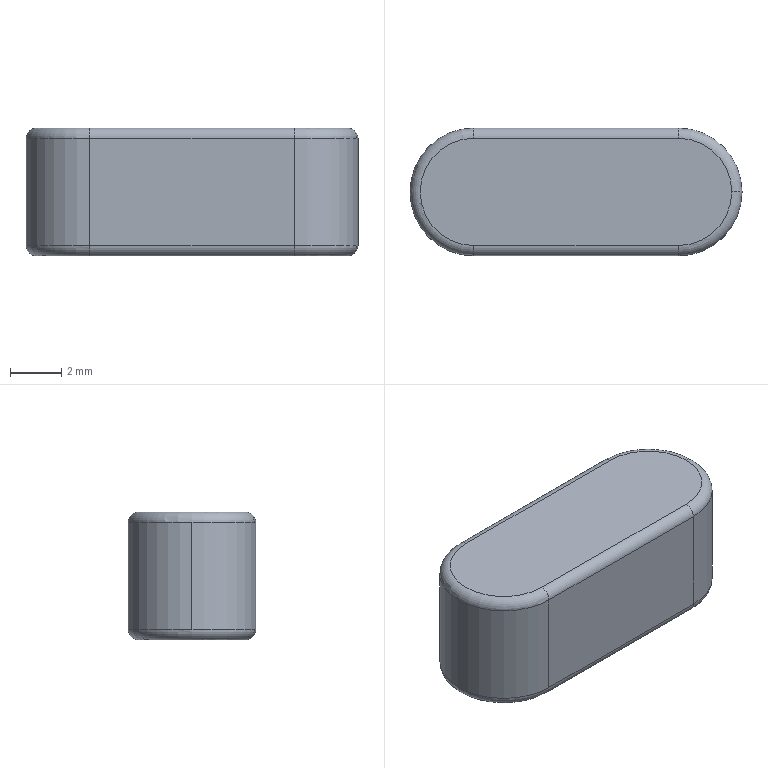Part | SolidWorks | features Extrusion 1, Fillet 1 | 1 solid | 17 faces | box 13 x 5 x 5 mm | volume 296.036 mm3 | cylinder 7 | torus 6 | plane 4 | commonest cylinder face diameters 0.8 x4 5 x3
STEP:
#1=CARTESIAN_POINT('',(6.1,0.,0.));
#2=VERTEX_POINT('',#1);
#3=CARTESIAN_POINT('',(4.,-2.1,0.));
#4=VERTEX_POINT('',#3);
#5=CARTESIAN_POINT('',(4.,0.,0.));
#6=DIRECTION('',(0.,0.,-1.));
#7=DIRECTION('',(1.,0.,0.));
#8=AXIS2_PLACEMENT_3D('',#5,#6,#7);
#9=CIRCLE('',#8,2.1);
#10=EDGE_CURVE('',#2,#4,#9,.T.);
#11=ORIENTED_EDGE('',*,*,#10,.F.);
#12=CARTESIAN_POINT('',(6.5,0.,0.4));
#13=VERTEX_POINT('',#12);
#14=CARTESIAN_POINT('',(6.1,0.,0.4));
#15=DIRECTION('',(0.,-1.,0.));
#16=DIRECTION('',(0.,0.,-1.));
#17=AXIS2_PLACEMENT_3D('',#14,#15,#16);
#18=CIRCLE('',#17,0.4);
#19=EDGE_CURVE('',#2,#13,#18,.T.);
#20=ORIENTED_EDGE('',*,*,#19,.T.);
#21=CARTESIAN_POINT('',(4.,-2.5,0.4));
#22=VERTEX_POINT('',#21);
#23=CARTESIAN_POINT('',(4.,0.,0.4));
#24=DIRECTION('',(0.,0.,1.));
#25=DIRECTION('',(1.,0.,0.));
#26=AXIS2_PLACEMENT_3D('',#23,#24,#25);
#27=CIRCLE('',#26,2.5);
#28=EDGE_CURVE('',#22,#13,#27,.T.);
#29=ORIENTED_EDGE('',*,*,#28,.F.);
#30=CARTESIAN_POINT('',(4.,-2.1,0.4));
#31=DIRECTION('',(1.,0.,0.));
#32=DIRECTION('',(0.,0.,-1.));
#33=AXIS2_PLACEMENT_3D('',#30,#31,#32);
#34=CIRCLE('',#33,0.4);
#35=EDGE_CURVE('',#22,#4,#34,.T.);
#36=ORIENTED_EDGE('',*,*,#35,.T.);
#37=EDGE_LOOP('',(#11,#20,#29,#36));
#38=FACE_OUTER_BOUND('',#37,.T.);
#39=CARTESIAN_POINT('',(4.,0.,0.4));
#40=DIRECTION('',(0.,0.,1.));
#41=DIRECTION('',(1.,0.,0.));
#42=AXIS2_PLACEMENT_3D('',#39,#40,#41);
#43=TOROIDAL_SURFACE('',#42,2.1,0.4);
#44=ADVANCED_FACE('',(#38),#43,.T.);
#45=CARTESIAN_POINT('',(6.5,0.,4.6));
#46=VERTEX_POINT('',#45);
#47=CARTESIAN_POINT('',(4.,-2.5,4.6));
#48=VERTEX_POINT('',#47);
#49=CARTESIAN_POINT('',(4.,0.,4.6));
#50=DIRECTION('',(0.,0.,-1.));
#51=DIRECTION('',(1.,0.,0.));
#52=AXIS2_PLACEMENT_3D('',#49,#50,#51);
#53=CIRCLE('',#52,2.5);
#54=EDGE_CURVE('',#46,#48,#53,.T.);
#55=ORIENTED_EDGE('',*,*,#54,.F.);
#56=CARTESIAN_POINT('',(6.1,0.,5.));
#57=VERTEX_POINT('',#56);
#58=CARTESIAN_POINT('',(6.1,0.,4.6));
#59=DIRECTION('',(0.,-1.,0.));
#60=DIRECTION('',(0.,0.,-1.));
#61=AXIS2_PLACEMENT_3D('',#58,#59,#60);
#62=CIRCLE('',#61,0.4);
#63=EDGE_CURVE('',#46,#57,#62,.T.);
#64=ORIENTED_EDGE('',*,*,#63,.T.);
#65=CARTESIAN_POINT('',(4.,-2.1,5.));
#66=VERTEX_POINT('',#65);
#67=CARTESIAN_POINT('',(4.,0.,5.));
#68=DIRECTION('',(0.,0.,1.));
#69=DIRECTION('',(1.,0.,0.));
#70=AXIS2_PLACEMENT_3D('',#67,#68,#69);
#71=CIRCLE('',#70,2.1);
#72=EDGE_CURVE('',#66,#57,#71,.T.);
#73=ORIENTED_EDGE('',*,*,#72,.F.);
#74=CARTESIAN_POINT('',(4.,-2.1,4.6));
#75=DIRECTION('',(1.,0.,0.));
#76=DIRECTION('',(0.,0.,-1.));
#77=AXIS2_PLACEMENT_3D('',#74,#75,#76);
#78=CIRCLE('',#77,0.4);
#79=EDGE_CURVE('',#66,#48,#78,.T.);
#80=ORIENTED_EDGE('',*,*,#79,.T.);
#81=EDGE_LOOP('',(#55,#64,#73,#80));
#82=FACE_OUTER_BOUND('',#81,.T.);
#83=CARTESIAN_POINT('',(4.,0.,4.6));
#84=DIRECTION('',(0.,0.,1.));
#85=DIRECTION('',(1.,0.,0.));
#86=AXIS2_PLACEMENT_3D('',#83,#84,#85);
#87=TOROIDAL_SURFACE('',#86,2.1,0.4);
#88=ADVANCED_FACE('',(#82),#87,.T.);
#89=CARTESIAN_POINT('',(-4.,-2.5,4.6));
#90=VERTEX_POINT('',#89);
#91=CARTESIAN_POINT('',(-6.5,0.,4.6));
#92=VERTEX_POINT('',#91);
#93=CARTESIAN_POINT('',(-4.,0.,4.6));
#94=DIRECTION('',(0.,0.,-1.));
#95=DIRECTION('',(1.,0.,0.));
#96=AXIS2_PLACEMENT_3D('',#93,#94,#95);
#97=CIRCLE('',#96,2.5);
#98=EDGE_CURVE('',#90,#92,#97,.T.);
#99=ORIENTED_EDGE('',*,*,#98,.T.);
#100=CARTESIAN_POINT('',(-6.5,0.,0.4));
#101=VERTEX_POINT('',#100);
#102=CARTESIAN_POINT('',(-6.5,0.,5.));
#103=DIRECTION('',(0.,0.,-1.));
#104=VECTOR('',#103,1000.);
#105=LINE('',#102,#104);
#106=EDGE_CURVE('',#92,#101,#105,.T.);
#107=ORIENTED_EDGE('',*,*,#106,.T.);
#108=CARTESIAN_POINT('',(-4.,-2.5,0.4));
#109=VERTEX_POINT('',#108);
#110=CARTESIAN_POINT('',(-4.,0.,0.4));
#111=DIRECTION('',(0.,0.,1.));
#112=DIRECTION('',(1.,0.,0.));
#113=AXIS2_PLACEMENT_3D('',#110,#111,#112);
#114=CIRCLE('',#113,2.5);
#115=EDGE_CURVE('',#101,#109,#114,.T.);
#116=ORIENTED_EDGE('',*,*,#115,.T.);
#117=CARTESIAN_POINT('',(-4.,-2.5,5.));
#118=DIRECTION('',(0.,0.,-1.));
#119=VECTOR('',#118,1000.);
#120=LINE('',#117,#119);
#121=EDGE_CURVE('',#90,#109,#120,.T.);
#122=ORIENTED_EDGE('',*,*,#121,.F.);
#123=EDGE_LOOP('',(#99,#107,#116,#122));
#124=FACE_OUTER_BOUND('',#123,.T.);
#125=CARTESIAN_POINT('',(-4.,0.,5.));
#126=DIRECTION('',(0.,0.,-1.));
#127=DIRECTION('',(-1.,0.,0.));
#128=AXIS2_PLACEMENT_3D('',#125,#126,#127);
#129=CYLINDRICAL_SURFACE('',#128,2.5);
#130=ADVANCED_FACE('',(#124),#129,.T.);
#131=ORIENTED_EDGE('',*,*,#106,.F.);
#132=CARTESIAN_POINT('',(-4.,2.5,4.6));
#133=VERTEX_POINT('',#132);
#134=CARTESIAN_POINT('',(-4.,0.,4.6));
#135=DIRECTION('',(0.,0.,-1.));
#136=DIRECTION('',(1.,0.,0.));
#137=AXIS2_PLACEMENT_3D('',#134,#135,#136);
#138=CIRCLE('',#137,2.5);
#139=EDGE_CURVE('',#92,#133,#138,.T.);
#140=ORIENTED_EDGE('',*,*,#139,.T.);
#141=CARTESIAN_POINT('',(-4.,2.5,0.4));
#142=VERTEX_POINT('',#141);
#143=CARTESIAN_POINT('',(-4.,2.5,5.));
#144=DIRECTION('',(0.,0.,-1.));
#145=VECTOR('',#144,1000.);
#146=LINE('',#143,#145);
#147=EDGE_CURVE('',#133,#142,#146,.T.);
#148=ORIENTED_EDGE('',*,*,#147,.T.);
#149=CARTESIAN_POINT('',(-4.,0.,0.4));
#150=DIRECTION('',(0.,0.,1.));
#151=DIRECTION('',(1.,0.,0.));
#152=AXIS2_PLACEMENT_3D('',#149,#150,#151);
#153=CIRCLE('',#152,2.5);
#154=EDGE_CURVE('',#142,#101,#153,.T.);
#155=ORIENTED_EDGE('',*,*,#154,.T.);
#156=EDGE_LOOP('',(#131,#140,#148,#155));
#157=FACE_OUTER_BOUND('',#156,.T.);
#158=CARTESIAN_POINT('',(-4.,0.,5.));
#159=DIRECTION('',(0.,0.,-1.));
#160=DIRECTION('',(-1.,0.,0.));
#161=AXIS2_PLACEMENT_3D('',#158,#159,#160);
#162=CYLINDRICAL_SURFACE('',#161,2.5);
#163=ADVANCED_FACE('',(#157),#162,.T.);
#164=CARTESIAN_POINT('',(4.,-2.5,5.));
#165=DIRECTION('',(0.,0.,-1.));
#166=VECTOR('',#165,1000.);
#167=LINE('',#164,#166);
#168=EDGE_CURVE('',#48,#22,#167,.T.);
#169=ORIENTED_EDGE('',*,*,#168,.F.);
#170=CARTESIAN_POINT('',(-4.,-2.5,4.6));
#171=DIRECTION('',(-1.,0.,0.));
#172=VECTOR('',#171,1000.);
#173=LINE('',#170,#172);
#174=EDGE_CURVE('',#48,#90,#173,.T.);
#175=ORIENTED_EDGE('',*,*,#174,.T.);
#176=ORIENTED_EDGE('',*,*,#121,.T.);
#177=CARTESIAN_POINT('',(-4.,-2.5,0.4));
#178=DIRECTION('',(1.,0.,0.));
#179=VECTOR('',#178,1000.);
#180=LINE('',#177,#179);
#181=EDGE_CURVE('',#109,#22,#180,.T.);
#182=ORIENTED_EDGE('',*,*,#181,.T.);
#183=EDGE_LOOP('',(#169,#175,#176,#182));
#184=FACE_OUTER_BOUND('',#183,.T.);
#185=CARTESIAN_POINT('',(-4.,-2.5,5.));
#186=DIRECTION('',(0.,1.,0.));
#187=DIRECTION('',(-1.,0.,0.));
#188=AXIS2_PLACEMENT_3D('',#185,#186,#187);
#189=PLANE('',#188);
#190=ADVANCED_FACE('',(#184),#189,.F.);
#191=CARTESIAN_POINT('',(4.,2.5,4.6));
#192=VERTEX_POINT('',#191);
#193=CARTESIAN_POINT('',(4.,2.5,0.4));
#194=VERTEX_POINT('',#193);
#195=CARTESIAN_POINT('',(4.,2.5,5.));
#196=DIRECTION('',(0.,0.,-1.));
#197=VECTOR('',#196,1000.);
#198=LINE('',#195,#197);
#199=EDGE_CURVE('',#192,#194,#198,.T.);
#200=ORIENTED_EDGE('',*,*,#199,.F.);
#201=CARTESIAN_POINT('',(4.,0.,4.6));
#202=DIRECTION('',(0.,0.,-1.));
#203=DIRECTION('',(1.,0.,0.));
#204=AXIS2_PLACEMENT_3D('',#201,#202,#203);
#205=CIRCLE('',#204,2.5);
#206=EDGE_CURVE('',#192,#46,#205,.T.);
#207=ORIENTED_EDGE('',*,*,#206,.T.);
#208=ORIENTED_EDGE('',*,*,#54,.T.);
#209=ORIENTED_EDGE('',*,*,#168,.T.);
#210=ORIENTED_EDGE('',*,*,#28,.T.);
#211=CARTESIAN_POINT('',(4.,0.,0.4));
#212=DIRECTION('',(0.,0.,1.));
#213=DIRECTION('',(1.,0.,0.));
#214=AXIS2_PLACEMENT_3D('',#211,#212,#213);
#215=CIRCLE('',#214,2.5);
#216=EDGE_CURVE('',#13,#194,#215,.T.);
#217=ORIENTED_EDGE('',*,*,#216,.T.);
#218=EDGE_LOOP('',(#200,#207,#208,#209,#210,#217));
#219=FACE_OUTER_BOUND('',#218,.T.);
#220=CARTESIAN_POINT('',(4.,0.,5.));
#221=DIRECTION('',(0.,0.,-1.));
#222=DIRECTION('',(-1.,0.,0.));
#223=AXIS2_PLACEMENT_3D('',#220,#221,#222);
#224=CYLINDRICAL_SURFACE('',#223,2.5);
#225=ADVANCED_FACE('',(#219),#224,.T.);
#226=ORIENTED_EDGE('',*,*,#147,.F.);
#227=CARTESIAN_POINT('',(4.,2.5,4.6));
#228=DIRECTION('',(1.,0.,0.));
#229=VECTOR('',#228,1000.);
#230=LINE('',#227,#229);
#231=EDGE_CURVE('',#133,#192,#230,.T.);
#232=ORIENTED_EDGE('',*,*,#231,.T.);
#233=ORIENTED_EDGE('',*,*,#199,.T.);
#234=CARTESIAN_POINT('',(-4.,2.5,0.4));
#235=DIRECTION('',(-1.,0.,0.));
#236=VECTOR('',#235,1000.);
#237=LINE('',#234,#236);
#238=EDGE_CURVE('',#194,#142,#237,.T.);
#239=ORIENTED_EDGE('',*,*,#238,.T.);
#240=EDGE_LOOP('',(#226,#232,#233,#239));
#241=FACE_OUTER_BOUND('',#240,.T.);
#242=CARTESIAN_POINT('',(-4.,2.5,5.));
#243=DIRECTION('',(0.,-1.,0.));
#244=DIRECTION('',(1.,0.,0.));
#245=AXIS2_PLACEMENT_3D('',#242,#243,#244);
#246=PLANE('',#245);
#247=ADVANCED_FACE('',(#241),#246,.F.);
#248=CARTESIAN_POINT('',(-4.,-2.1,5.));
#249=VERTEX_POINT('',#248);
#250=CARTESIAN_POINT('',(4.,-2.1,5.));
#251=DIRECTION('',(1.,0.,0.));
#252=VECTOR('',#251,1000.);
#253=LINE('',#250,#252);
#254=EDGE_CURVE('',#249,#66,#253,.T.);
#255=ORIENTED_EDGE('',*,*,#254,.T.);
#256=ORIENTED_EDGE('',*,*,#72,.T.);
#257=CARTESIAN_POINT('',(4.,2.1,5.));
#258=VERTEX_POINT('',#257);
#259=CARTESIAN_POINT('',(4.,0.,5.));
#260=DIRECTION('',(0.,0.,1.));
#261=DIRECTION('',(1.,0.,0.));
#262=AXIS2_PLACEMENT_3D('',#259,#260,#261);
#263=CIRCLE('',#262,2.1);
#264=EDGE_CURVE('',#57,#258,#263,.T.);
#265=ORIENTED_EDGE('',*,*,#264,.T.);
#266=CARTESIAN_POINT('',(-4.,2.1,5.));
#267=VERTEX_POINT('',#266);
#268=CARTESIAN_POINT('',(-4.,2.1,5.));
#269=DIRECTION('',(-1.,0.,0.));
#270=VECTOR('',#269,1000.);
#271=LINE('',#268,#270);
#272=EDGE_CURVE('',#258,#267,#271,.T.);
#273=ORIENTED_EDGE('',*,*,#272,.T.);
#274=CARTESIAN_POINT('',(-4.,0.,5.));
#275=DIRECTION('',(0.,0.,1.));
#276=DIRECTION('',(1.,0.,0.));
#277=AXIS2_PLACEMENT_3D('',#274,#275,#276);
#278=CIRCLE('',#277,2.1);
#279=EDGE_CURVE('',#267,#249,#278,.T.);
#280=ORIENTED_EDGE('',*,*,#279,.T.);
#281=EDGE_LOOP('',(#255,#256,#265,#273,#280));
#282=FACE_OUTER_BOUND('',#281,.T.);
#283=CARTESIAN_POINT('',(-4.,0.,5.));
#284=DIRECTION('',(0.,0.,1.));
#285=DIRECTION('',(1.,0.,0.));
#286=AXIS2_PLACEMENT_3D('',#283,#284,#285);
#287=PLANE('',#286);
#288=ADVANCED_FACE('',(#282),#287,.T.);
#289=CARTESIAN_POINT('',(-4.,2.1,0.));
#290=VERTEX_POINT('',#289);
#291=CARTESIAN_POINT('',(4.,2.1,0.));
#292=VERTEX_POINT('',#291);
#293=CARTESIAN_POINT('',(-4.,2.1,0.));
#294=DIRECTION('',(1.,0.,0.));
#295=VECTOR('',#294,1000.);
#296=LINE('',#293,#295);
#297=EDGE_CURVE('',#290,#292,#296,.T.);
#298=ORIENTED_EDGE('',*,*,#297,.T.);
#299=CARTESIAN_POINT('',(4.,0.,0.));
#300=DIRECTION('',(0.,0.,-1.));
#301=DIRECTION('',(1.,0.,0.));
#302=AXIS2_PLACEMENT_3D('',#299,#300,#301);
#303=CIRCLE('',#302,2.1);
#304=EDGE_CURVE('',#292,#2,#303,.T.);
#305=ORIENTED_EDGE('',*,*,#304,.T.);
#306=ORIENTED_EDGE('',*,*,#10,.T.);
#307=CARTESIAN_POINT('',(-4.,-2.1,0.));
#308=VERTEX_POINT('',#307);
#309=CARTESIAN_POINT('',(-4.,-2.1,0.));
#310=DIRECTION('',(-1.,0.,0.));
#311=VECTOR('',#310,1000.);
#312=LINE('',#309,#311);
#313=EDGE_CURVE('',#4,#308,#312,.T.);
#314=ORIENTED_EDGE('',*,*,#313,.T.);
#315=CARTESIAN_POINT('',(-4.,0.,0.));
#316=DIRECTION('',(0.,0.,-1.));
#317=DIRECTION('',(1.,0.,0.));
#318=AXIS2_PLACEMENT_3D('',#315,#316,#317);
#319=CIRCLE('',#318,2.1);
#320=EDGE_CURVE('',#308,#290,#319,.T.);
#321=ORIENTED_EDGE('',*,*,#320,.T.);
#322=EDGE_LOOP('',(#298,#305,#306,#314,#321));
#323=FACE_OUTER_BOUND('',#322,.T.);
#324=CARTESIAN_POINT('',(-4.,0.,0.));
#325=DIRECTION('',(0.,0.,1.));
#326=DIRECTION('',(1.,0.,0.));
#327=AXIS2_PLACEMENT_3D('',#324,#325,#326);
#328=PLANE('',#327);
#329=ADVANCED_FACE('',(#323),#328,.F.);
#330=CARTESIAN_POINT('',(-4.,2.1,4.6));
#331=DIRECTION('',(1.,0.,0.));
#332=DIRECTION('',(0.,0.,-1.));
#333=AXIS2_PLACEMENT_3D('',#330,#331,#332);
#334=CIRCLE('',#333,0.4);
#335=EDGE_CURVE('',#133,#267,#334,.T.);
#336=ORIENTED_EDGE('',*,*,#335,.F.);
#337=ORIENTED_EDGE('',*,*,#139,.F.);
#338=ORIENTED_EDGE('',*,*,#98,.F.);
#339=CARTESIAN_POINT('',(-4.,-2.1,4.6));
#340=DIRECTION('',(1.,0.,0.));
#341=DIRECTION('',(0.,0.,-1.));
#342=AXIS2_PLACEMENT_3D('',#339,#340,#341);
#343=CIRCLE('',#342,0.4);
#344=EDGE_CURVE('',#249,#90,#343,.T.);
#345=ORIENTED_EDGE('',*,*,#344,.F.);
#346=ORIENTED_EDGE('',*,*,#279,.F.);
#347=EDGE_LOOP('',(#336,#337,#338,#345,#346));
#348=FACE_OUTER_BOUND('',#347,.T.);
#349=CARTESIAN_POINT('',(-4.,0.,4.6));
#350=DIRECTION('',(0.,0.,1.));
#351=DIRECTION('',(1.,0.,0.));
#352=AXIS2_PLACEMENT_3D('',#349,#350,#351);
#353=TOROIDAL_SURFACE('',#352,2.1,0.4);
#354=ADVANCED_FACE('',(#348),#353,.T.);
#355=ORIENTED_EDGE('',*,*,#344,.T.);
#356=ORIENTED_EDGE('',*,*,#174,.F.);
#357=ORIENTED_EDGE('',*,*,#79,.F.);
#358=ORIENTED_EDGE('',*,*,#254,.F.);
#359=EDGE_LOOP('',(#355,#356,#357,#358));
#360=FACE_OUTER_BOUND('',#359,.T.);
#361=CARTESIAN_POINT('',(-4.,-2.1,4.6));
#362=DIRECTION('',(-1.,0.,0.));
#363=DIRECTION('',(0.,-1.,0.));
#364=AXIS2_PLACEMENT_3D('',#361,#362,#363);
#365=CYLINDRICAL_SURFACE('',#364,0.4);
#366=ADVANCED_FACE('',(#360),#365,.T.);
#367=ORIENTED_EDGE('',*,*,#335,.T.);
#368=ORIENTED_EDGE('',*,*,#272,.F.);
#369=CARTESIAN_POINT('',(4.,2.1,4.6));
#370=DIRECTION('',(1.,0.,0.));
#371=DIRECTION('',(0.,0.,-1.));
#372=AXIS2_PLACEMENT_3D('',#369,#370,#371);
#373=CIRCLE('',#372,0.4);
#374=EDGE_CURVE('',#192,#258,#373,.T.);
#375=ORIENTED_EDGE('',*,*,#374,.F.);
#376=ORIENTED_EDGE('',*,*,#231,.F.);
#377=EDGE_LOOP('',(#367,#368,#375,#376));
#378=FACE_OUTER_BOUND('',#377,.T.);
#379=CARTESIAN_POINT('',(-4.,2.1,4.6));
#380=DIRECTION('',(1.,0.,0.));
#381=DIRECTION('',(0.,1.,0.));
#382=AXIS2_PLACEMENT_3D('',#379,#380,#381);
#383=CYLINDRICAL_SURFACE('',#382,0.4);
#384=ADVANCED_FACE('',(#378),#383,.T.);
#385=ORIENTED_EDGE('',*,*,#63,.F.);
#386=ORIENTED_EDGE('',*,*,#206,.F.);
#387=ORIENTED_EDGE('',*,*,#374,.T.);
#388=ORIENTED_EDGE('',*,*,#264,.F.);
#389=EDGE_LOOP('',(#385,#386,#387,#388));
#390=FACE_OUTER_BOUND('',#389,.T.);
#391=CARTESIAN_POINT('',(4.,0.,4.6));
#392=DIRECTION('',(0.,0.,1.));
#393=DIRECTION('',(1.,0.,0.));
#394=AXIS2_PLACEMENT_3D('',#391,#392,#393);
#395=TOROIDAL_SURFACE('',#394,2.1,0.4);
#396=ADVANCED_FACE('',(#390),#395,.T.);
#397=CARTESIAN_POINT('',(-4.,2.1,0.4));
#398=DIRECTION('',(1.,0.,0.));
#399=DIRECTION('',(0.,0.,-1.));
#400=AXIS2_PLACEMENT_3D('',#397,#398,#399);
#401=CIRCLE('',#400,0.4);
#402=EDGE_CURVE('',#290,#142,#401,.T.);
#403=ORIENTED_EDGE('',*,*,#402,.F.);
#404=ORIENTED_EDGE('',*,*,#320,.F.);
#405=CARTESIAN_POINT('',(-4.,-2.1,0.4));
#406=DIRECTION('',(1.,0.,0.));
#407=DIRECTION('',(0.,0.,-1.));
#408=AXIS2_PLACEMENT_3D('',#405,#406,#407);
#409=CIRCLE('',#408,0.4);
#410=EDGE_CURVE('',#109,#308,#409,.T.);
#411=ORIENTED_EDGE('',*,*,#410,.F.);
#412=ORIENTED_EDGE('',*,*,#115,.F.);
#413=ORIENTED_EDGE('',*,*,#154,.F.);
#414=EDGE_LOOP('',(#403,#404,#411,#412,#413));
#415=FACE_OUTER_BOUND('',#414,.T.);
#416=CARTESIAN_POINT('',(-4.,0.,0.4));
#417=DIRECTION('',(0.,0.,1.));
#418=DIRECTION('',(1.,0.,0.));
#419=AXIS2_PLACEMENT_3D('',#416,#417,#418);
#420=TOROIDAL_SURFACE('',#419,2.1,0.4);
#421=ADVANCED_FACE('',(#415),#420,.T.);
#422=ORIENTED_EDGE('',*,*,#410,.T.);
#423=ORIENTED_EDGE('',*,*,#313,.F.);
#424=ORIENTED_EDGE('',*,*,#35,.F.);
#425=ORIENTED_EDGE('',*,*,#181,.F.);
#426=EDGE_LOOP('',(#422,#423,#424,#425));
#427=FACE_OUTER_BOUND('',#426,.T.);
#428=CARTESIAN_POINT('',(-4.,-2.1,0.4));
#429=DIRECTION('',(1.,0.,0.));
#430=DIRECTION('',(0.,1.,0.));
#431=AXIS2_PLACEMENT_3D('',#428,#429,#430);
#432=CYLINDRICAL_SURFACE('',#431,0.4);
#433=ADVANCED_FACE('',(#427),#432,.T.);
#434=ORIENTED_EDGE('',*,*,#402,.T.);
#435=ORIENTED_EDGE('',*,*,#238,.F.);
#436=CARTESIAN_POINT('',(4.,2.1,0.4));
#437=DIRECTION('',(1.,0.,0.));
#438=DIRECTION('',(0.,0.,-1.));
#439=AXIS2_PLACEMENT_3D('',#436,#437,#438);
#440=CIRCLE('',#439,0.4);
#441=EDGE_CURVE('',#292,#194,#440,.T.);
#442=ORIENTED_EDGE('',*,*,#441,.F.);
#443=ORIENTED_EDGE('',*,*,#297,.F.);
#444=EDGE_LOOP('',(#434,#435,#442,#443));
#445=FACE_OUTER_BOUND('',#444,.T.);
#446=CARTESIAN_POINT('',(-4.,2.1,0.4));
#447=DIRECTION('',(-1.,0.,0.));
#448=DIRECTION('',(0.,-1.,0.));
#449=AXIS2_PLACEMENT_3D('',#446,#447,#448);
#450=CYLINDRICAL_SURFACE('',#449,0.4);
#451=ADVANCED_FACE('',(#445),#450,.T.);
#452=ORIENTED_EDGE('',*,*,#19,.F.);
#453=ORIENTED_EDGE('',*,*,#304,.F.);
#454=ORIENTED_EDGE('',*,*,#441,.T.);
#455=ORIENTED_EDGE('',*,*,#216,.F.);
#456=EDGE_LOOP('',(#452,#453,#454,#455));
#457=FACE_OUTER_BOUND('',#456,.T.);
#458=CARTESIAN_POINT('',(4.,0.,0.4));
#459=DIRECTION('',(0.,0.,1.));
#460=DIRECTION('',(1.,0.,0.));
#461=AXIS2_PLACEMENT_3D('',#458,#459,#460);
#462=TOROIDAL_SURFACE('',#461,2.1,0.4);
#463=ADVANCED_FACE('',(#457),#462,.T.);
#464=CLOSED_SHELL('',(#44,#88,#130,#163,#190,#225,#247,#288,#329,#354,#366,#384,#396,#421,#433,#451,#463));
#465=MANIFOLD_SOLID_BREP('',#464);
#466=CARTESIAN_POINT('',(0.,0.,0.));
#467=DIRECTION('',(0.,0.,1.));
#468=DIRECTION('',(1.,0.,0.));
#469=AXIS2_PLACEMENT_3D('',#466,#467,#468);
#470=(LENGTH_UNIT()NAMED_UNIT(*)SI_UNIT(.MILLI.,.METRE.));
#471=UNCERTAINTY_MEASURE_WITH_UNIT(LENGTH_MEASURE(0.00001),#470,'','');
#472=(NAMED_UNIT(*)PLANE_ANGLE_UNIT()SI_UNIT($,.RADIAN.));
#473=(NAMED_UNIT(*)SI_UNIT($,.STERADIAN.)SOLID_ANGLE_UNIT());
#474=(GEOMETRIC_REPRESENTATION_CONTEXT(3)GLOBAL_UNCERTAINTY_ASSIGNED_CONTEXT((#471))GLOBAL_UNIT_ASSIGNED_CONTEXT((#470,#472,#473))REPRESENTATION_CONTEXT('',''));
#475=ADVANCED_BREP_SHAPE_REPRESENTATION('',(#465,#469),#474);